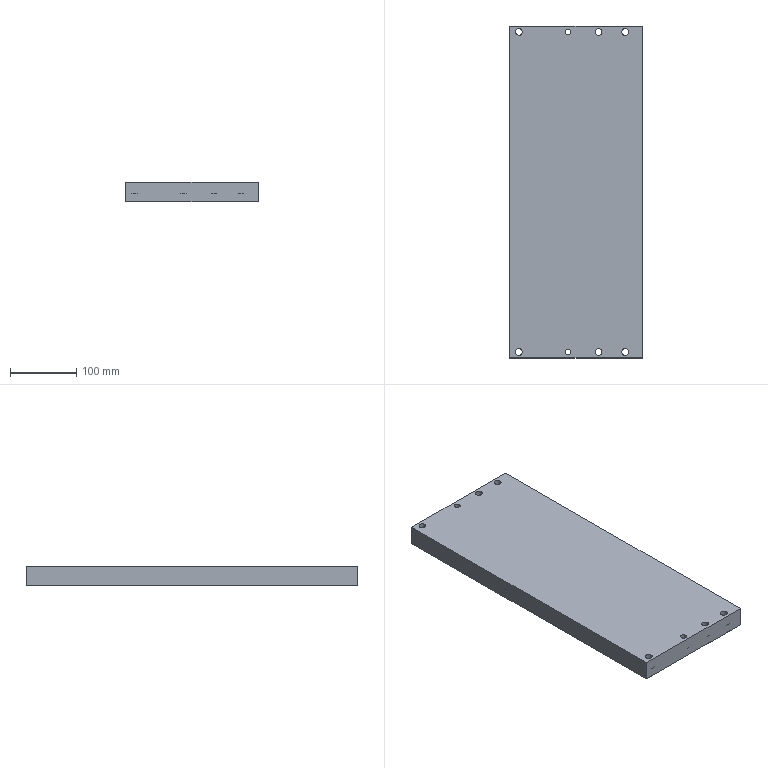Part | NX | 1 solid | 30 faces | box 200 x 500 x 30 mm | volume 2965920 mm3 | cylinder 16 | plane 14 | commonest cylinder face diameters 17 x8 10.3 x6 8.6 x2
STEP:
#1=CARTESIAN_POINT('',(-86.,-483.5,-60.));
#2=VERTEX_POINT('',#1);
#3=CARTESIAN_POINT('',(-86.,-492.,-60.));
#4=DIRECTION('',(0.,0.,-1.));
#5=DIRECTION('',(0.,1.,0.));
#6=AXIS2_PLACEMENT_3D('',#3,#4,#5);
#7=CIRCLE('',#6,8.5);
#8=EDGE_CURVE('',#2,#2,#7,.T.);
#9=ORIENTED_EDGE('',*,*,#8,.F.);
#10=EDGE_LOOP('',(#9));
#11=FACE_BOUND('',#10,.T.);
#12=CARTESIAN_POINT('',(-94.5,-492.,-73.));
#13=VERTEX_POINT('',#12);
#14=CARTESIAN_POINT('',(-86.,-492.,-73.));
#15=DIRECTION('',(0.,0.,-1.));
#16=DIRECTION('',(-1.,0.,0.));
#17=AXIS2_PLACEMENT_3D('',#14,#15,#16);
#18=CIRCLE('',#17,8.5);
#19=EDGE_CURVE('',#13,#13,#18,.F.);
#20=ORIENTED_EDGE('',*,*,#19,.F.);
#21=EDGE_LOOP('',(#20));
#22=FACE_BOUND('',#21,.T.);
#23=CARTESIAN_POINT('',(-86.,-492.,-60.));
#24=DIRECTION('',(0.,0.,-1.));
#25=DIRECTION('',(-1.,0.,0.));
#26=AXIS2_PLACEMENT_3D('',#23,#24,#25);
#27=CYLINDRICAL_SURFACE('',#26,8.5);
#28=ADVANCED_FACE('',(#11,#22),#27,.F.);
#29=ORIENTED_EDGE('',*,*,#8,.T.);
#30=EDGE_LOOP('',(#29));
#31=FACE_BOUND('',#30,.T.);
#32=CARTESIAN_POINT('',(-80.85,-492.,-60.));
#33=VERTEX_POINT('',#32);
#34=CARTESIAN_POINT('',(-86.,-492.,-60.));
#35=DIRECTION('',(0.,0.,-1.));
#36=DIRECTION('',(1.,0.,0.));
#37=AXIS2_PLACEMENT_3D('',#34,#35,#36);
#38=CIRCLE('',#37,5.15);
#39=EDGE_CURVE('',#33,#33,#38,.T.);
#40=ORIENTED_EDGE('',*,*,#39,.F.);
#41=EDGE_LOOP('',(#40));
#42=FACE_BOUND('',#41,.T.);
#43=CARTESIAN_POINT('',(-86.,-492.,-60.));
#44=DIRECTION('',(0.,0.,1.));
#45=DIRECTION('',(1.,0.,0.));
#46=AXIS2_PLACEMENT_3D('',#43,#44,#45);
#47=PLANE('',#46);
#48=ADVANCED_FACE('',(#31,#42),#47,.F.);
#49=ORIENTED_EDGE('',*,*,#39,.T.);
#50=EDGE_LOOP('',(#49));
#51=FACE_BOUND('',#50,.T.);
#52=CARTESIAN_POINT('',(-80.85,-492.,-43.));
#53=VERTEX_POINT('',#52);
#54=CARTESIAN_POINT('',(-86.,-492.,-43.));
#55=DIRECTION('',(0.,0.,1.));
#56=DIRECTION('',(1.,0.,0.));
#57=AXIS2_PLACEMENT_3D('',#54,#55,#56);
#58=CIRCLE('',#57,5.15);
#59=EDGE_CURVE('',#53,#53,#58,.T.);
#60=ORIENTED_EDGE('',*,*,#59,.T.);
#61=EDGE_LOOP('',(#60));
#62=FACE_BOUND('',#61,.T.);
#63=CARTESIAN_POINT('',(-86.,-492.,-78.));
#64=DIRECTION('',(0.,0.,1.));
#65=DIRECTION('',(1.,0.,0.));
#66=AXIS2_PLACEMENT_3D('',#63,#64,#65);
#67=CYLINDRICAL_SURFACE('',#66,5.15);
#68=ADVANCED_FACE('',(#51,#62),#67,.F.);
#69=CARTESIAN_POINT('',(79.15,-492.,-43.));
#70=VERTEX_POINT('',#69);
#71=CARTESIAN_POINT('',(74.,-492.,-43.));
#72=DIRECTION('',(0.,0.,1.));
#73=DIRECTION('',(1.,0.,0.));
#74=AXIS2_PLACEMENT_3D('',#71,#72,#73);
#75=CIRCLE('',#74,5.15);
#76=EDGE_CURVE('',#70,#70,#75,.F.);
#77=ORIENTED_EDGE('',*,*,#76,.F.);
#78=EDGE_LOOP('',(#77));
#79=FACE_BOUND('',#78,.T.);
#80=CARTESIAN_POINT('',(68.85,-492.,-60.));
#81=VERTEX_POINT('',#80);
#82=CARTESIAN_POINT('',(74.,-492.,-60.));
#83=DIRECTION('',(0.,0.,1.));
#84=DIRECTION('',(-1.,0.,0.));
#85=AXIS2_PLACEMENT_3D('',#82,#83,#84);
#86=CIRCLE('',#85,5.15);
#87=EDGE_CURVE('',#81,#81,#86,.F.);
#88=ORIENTED_EDGE('',*,*,#87,.T.);
#89=EDGE_LOOP('',(#88));
#90=FACE_BOUND('',#89,.T.);
#91=CARTESIAN_POINT('',(74.,-492.,-78.));
#92=DIRECTION('',(0.,0.,1.));
#93=DIRECTION('',(1.,0.,0.));
#94=AXIS2_PLACEMENT_3D('',#91,#92,#93);
#95=CYLINDRICAL_SURFACE('',#94,5.15);
#96=ADVANCED_FACE('',(#79,#90),#95,.F.);
#97=ORIENTED_EDGE('',*,*,#87,.F.);
#98=EDGE_LOOP('',(#97));
#99=FACE_BOUND('',#98,.T.);
#100=CARTESIAN_POINT('',(74.,-483.5,-60.));
#101=VERTEX_POINT('',#100);
#102=CARTESIAN_POINT('',(74.,-492.,-60.));
#103=DIRECTION('',(0.,0.,1.));
#104=DIRECTION('',(0.,1.,0.));
#105=AXIS2_PLACEMENT_3D('',#102,#103,#104);
#106=CIRCLE('',#105,8.5);
#107=EDGE_CURVE('',#101,#101,#106,.T.);
#108=ORIENTED_EDGE('',*,*,#107,.F.);
#109=EDGE_LOOP('',(#108));
#110=FACE_BOUND('',#109,.T.);
#111=CARTESIAN_POINT('',(74.,-492.,-60.));
#112=DIRECTION('',(0.,0.,-1.));
#113=DIRECTION('',(-1.,0.,0.));
#114=AXIS2_PLACEMENT_3D('',#111,#112,#113);
#115=PLANE('',#114);
#116=ADVANCED_FACE('',(#99,#110),#115,.T.);
#117=ORIENTED_EDGE('',*,*,#107,.T.);
#118=EDGE_LOOP('',(#117));
#119=FACE_BOUND('',#118,.T.);
#120=CARTESIAN_POINT('',(65.5,-492.,-73.));
#121=VERTEX_POINT('',#120);
#122=CARTESIAN_POINT('',(74.,-492.,-73.));
#123=DIRECTION('',(0.,0.,-1.));
#124=DIRECTION('',(-1.,0.,0.));
#125=AXIS2_PLACEMENT_3D('',#122,#123,#124);
#126=CIRCLE('',#125,8.5);
#127=EDGE_CURVE('',#121,#121,#126,.T.);
#128=ORIENTED_EDGE('',*,*,#127,.T.);
#129=EDGE_LOOP('',(#128));
#130=FACE_BOUND('',#129,.T.);
#131=CARTESIAN_POINT('',(74.,-492.,-60.));
#132=DIRECTION('',(0.,0.,-1.));
#133=DIRECTION('',(-1.,0.,0.));
#134=AXIS2_PLACEMENT_3D('',#131,#132,#133);
#135=CYLINDRICAL_SURFACE('',#134,8.5);
#136=ADVANCED_FACE('',(#119,#130),#135,.F.);
#137=CARTESIAN_POINT('',(39.15,-492.,-43.));
#138=VERTEX_POINT('',#137);
#139=CARTESIAN_POINT('',(34.,-492.,-43.));
#140=DIRECTION('',(0.,0.,1.));
#141=DIRECTION('',(1.,0.,0.));
#142=AXIS2_PLACEMENT_3D('',#139,#140,#141);
#143=CIRCLE('',#142,5.15);
#144=EDGE_CURVE('',#138,#138,#143,.F.);
#145=ORIENTED_EDGE('',*,*,#144,.F.);
#146=EDGE_LOOP('',(#145));
#147=FACE_BOUND('',#146,.T.);
#148=CARTESIAN_POINT('',(28.85,-492.,-60.));
#149=VERTEX_POINT('',#148);
#150=CARTESIAN_POINT('',(34.,-492.,-60.));
#151=DIRECTION('',(0.,0.,1.));
#152=DIRECTION('',(-1.,0.,0.));
#153=AXIS2_PLACEMENT_3D('',#150,#151,#152);
#154=CIRCLE('',#153,5.15);
#155=EDGE_CURVE('',#149,#149,#154,.F.);
#156=ORIENTED_EDGE('',*,*,#155,.T.);
#157=EDGE_LOOP('',(#156));
#158=FACE_BOUND('',#157,.T.);
#159=CARTESIAN_POINT('',(34.,-492.,-78.));
#160=DIRECTION('',(0.,0.,1.));
#161=DIRECTION('',(1.,0.,0.));
#162=AXIS2_PLACEMENT_3D('',#159,#160,#161);
#163=CYLINDRICAL_SURFACE('',#162,5.15);
#164=ADVANCED_FACE('',(#147,#158),#163,.F.);
#165=ORIENTED_EDGE('',*,*,#155,.F.);
#166=EDGE_LOOP('',(#165));
#167=FACE_BOUND('',#166,.T.);
#168=CARTESIAN_POINT('',(34.,-483.5,-60.));
#169=VERTEX_POINT('',#168);
#170=CARTESIAN_POINT('',(34.,-492.,-60.));
#171=DIRECTION('',(0.,0.,1.));
#172=DIRECTION('',(0.,1.,0.));
#173=AXIS2_PLACEMENT_3D('',#170,#171,#172);
#174=CIRCLE('',#173,8.5);
#175=EDGE_CURVE('',#169,#169,#174,.T.);
#176=ORIENTED_EDGE('',*,*,#175,.F.);
#177=EDGE_LOOP('',(#176));
#178=FACE_BOUND('',#177,.T.);
#179=CARTESIAN_POINT('',(34.,-492.,-60.));
#180=DIRECTION('',(0.,0.,-1.));
#181=DIRECTION('',(-1.,0.,0.));
#182=AXIS2_PLACEMENT_3D('',#179,#180,#181);
#183=PLANE('',#182);
#184=ADVANCED_FACE('',(#167,#178),#183,.T.);
#185=ORIENTED_EDGE('',*,*,#175,.T.);
#186=EDGE_LOOP('',(#185));
#187=FACE_BOUND('',#186,.T.);
#188=CARTESIAN_POINT('',(25.5,-492.,-73.));
#189=VERTEX_POINT('',#188);
#190=CARTESIAN_POINT('',(34.,-492.,-73.));
#191=DIRECTION('',(0.,0.,-1.));
#192=DIRECTION('',(-1.,0.,0.));
#193=AXIS2_PLACEMENT_3D('',#190,#191,#192);
#194=CIRCLE('',#193,8.5);
#195=EDGE_CURVE('',#189,#189,#194,.T.);
#196=ORIENTED_EDGE('',*,*,#195,.T.);
#197=EDGE_LOOP('',(#196));
#198=FACE_BOUND('',#197,.T.);
#199=CARTESIAN_POINT('',(34.,-492.,-60.));
#200=DIRECTION('',(0.,0.,-1.));
#201=DIRECTION('',(-1.,0.,0.));
#202=AXIS2_PLACEMENT_3D('',#199,#200,#201);
#203=CYLINDRICAL_SURFACE('',#202,8.5);
#204=ADVANCED_FACE('',(#187,#198),#203,.F.);
#205=CARTESIAN_POINT('',(-7.7,-492.,-43.));
#206=VERTEX_POINT('',#205);
#207=CARTESIAN_POINT('',(-12.,-492.,-43.));
#208=DIRECTION('',(0.,0.,1.));
#209=DIRECTION('',(1.,0.,0.));
#210=AXIS2_PLACEMENT_3D('',#207,#208,#209);
#211=CIRCLE('',#210,4.3);
#212=EDGE_CURVE('',#206,#206,#211,.F.);
#213=ORIENTED_EDGE('',*,*,#212,.F.);
#214=EDGE_LOOP('',(#213));
#215=FACE_BOUND('',#214,.T.);
#216=CARTESIAN_POINT('',(-16.3,-492.,-60.));
#217=VERTEX_POINT('',#216);
#218=CARTESIAN_POINT('',(-12.,-492.,-60.));
#219=DIRECTION('',(0.,0.,1.));
#220=DIRECTION('',(-1.,0.,0.));
#221=AXIS2_PLACEMENT_3D('',#218,#219,#220);
#222=CIRCLE('',#221,4.3);
#223=EDGE_CURVE('',#217,#217,#222,.F.);
#224=ORIENTED_EDGE('',*,*,#223,.T.);
#225=EDGE_LOOP('',(#224));
#226=FACE_BOUND('',#225,.T.);
#227=CARTESIAN_POINT('',(-12.,-492.,-78.));
#228=DIRECTION('',(0.,0.,1.));
#229=DIRECTION('',(1.,0.,0.));
#230=AXIS2_PLACEMENT_3D('',#227,#228,#229);
#231=CYLINDRICAL_SURFACE('',#230,4.3);
#232=ADVANCED_FACE('',(#215,#226),#231,.F.);
#233=ORIENTED_EDGE('',*,*,#223,.F.);
#234=EDGE_LOOP('',(#233));
#235=FACE_BOUND('',#234,.T.);
#236=CARTESIAN_POINT('',(-12.,-483.5,-60.));
#237=VERTEX_POINT('',#236);
#238=CARTESIAN_POINT('',(-12.,-492.,-60.));
#239=DIRECTION('',(0.,0.,1.));
#240=DIRECTION('',(0.,1.,0.));
#241=AXIS2_PLACEMENT_3D('',#238,#239,#240);
#242=CIRCLE('',#241,8.5);
#243=EDGE_CURVE('',#237,#237,#242,.T.);
#244=ORIENTED_EDGE('',*,*,#243,.F.);
#245=EDGE_LOOP('',(#244));
#246=FACE_BOUND('',#245,.T.);
#247=CARTESIAN_POINT('',(-12.,-492.,-60.));
#248=DIRECTION('',(0.,0.,-1.));
#249=DIRECTION('',(-1.,0.,0.));
#250=AXIS2_PLACEMENT_3D('',#247,#248,#249);
#251=PLANE('',#250);
#252=ADVANCED_FACE('',(#235,#246),#251,.T.);
#253=ORIENTED_EDGE('',*,*,#243,.T.);
#254=EDGE_LOOP('',(#253));
#255=FACE_BOUND('',#254,.T.);
#256=CARTESIAN_POINT('',(-20.5,-492.,-73.));
#257=VERTEX_POINT('',#256);
#258=CARTESIAN_POINT('',(-12.,-492.,-73.));
#259=DIRECTION('',(0.,0.,-1.));
#260=DIRECTION('',(-1.,0.,0.));
#261=AXIS2_PLACEMENT_3D('',#258,#259,#260);
#262=CIRCLE('',#261,8.5);
#263=EDGE_CURVE('',#257,#257,#262,.T.);
#264=ORIENTED_EDGE('',*,*,#263,.T.);
#265=EDGE_LOOP('',(#264));
#266=FACE_BOUND('',#265,.T.);
#267=CARTESIAN_POINT('',(-12.,-492.,-60.));
#268=DIRECTION('',(0.,0.,-1.));
#269=DIRECTION('',(-1.,0.,0.));
#270=AXIS2_PLACEMENT_3D('',#267,#268,#269);
#271=CYLINDRICAL_SURFACE('',#270,8.5);
#272=ADVANCED_FACE('',(#255,#266),#271,.F.);
#273=CARTESIAN_POINT('',(28.85,-10.,-60.));
#274=VERTEX_POINT('',#273);
#275=CARTESIAN_POINT('',(34.,-10.,-60.));
#276=DIRECTION('',(0.,0.,-1.));
#277=DIRECTION('',(-1.,0.,0.));
#278=AXIS2_PLACEMENT_3D('',#275,#276,#277);
#279=CIRCLE('',#278,5.15);
#280=EDGE_CURVE('',#274,#274,#279,.T.);
#281=ORIENTED_EDGE('',*,*,#280,.F.);
#282=EDGE_LOOP('',(#281));
#283=FACE_BOUND('',#282,.T.);
#284=CARTESIAN_POINT('',(34.,-18.5,-60.));
#285=VERTEX_POINT('',#284);
#286=CARTESIAN_POINT('',(34.,-10.,-60.));
#287=DIRECTION('',(0.,0.,-1.));
#288=DIRECTION('',(0.,-1.,0.));
#289=AXIS2_PLACEMENT_3D('',#286,#287,#288);
#290=CIRCLE('',#289,8.5);
#291=EDGE_CURVE('',#285,#285,#290,.F.);
#292=ORIENTED_EDGE('',*,*,#291,.F.);
#293=EDGE_LOOP('',(#292));
#294=FACE_BOUND('',#293,.T.);
#295=CARTESIAN_POINT('',(34.,-10.,-60.));
#296=DIRECTION('',(0.,0.,-1.));
#297=DIRECTION('',(-1.,0.,0.));
#298=AXIS2_PLACEMENT_3D('',#295,#296,#297);
#299=PLANE('',#298);
#300=ADVANCED_FACE('',(#283,#294),#299,.T.);
#301=CARTESIAN_POINT('',(-86.,-18.5,-60.));
#302=VERTEX_POINT('',#301);
#303=CARTESIAN_POINT('',(-86.,-10.,-60.));
#304=DIRECTION('',(0.,0.,1.));
#305=DIRECTION('',(0.,-1.,0.));
#306=AXIS2_PLACEMENT_3D('',#303,#304,#305);
#307=CIRCLE('',#306,8.5);
#308=EDGE_CURVE('',#302,#302,#307,.F.);
#309=ORIENTED_EDGE('',*,*,#308,.T.);
#310=EDGE_LOOP('',(#309));
#311=FACE_BOUND('',#310,.T.);
#312=CARTESIAN_POINT('',(-80.85,-10.,-60.));
#313=VERTEX_POINT('',#312);
#314=CARTESIAN_POINT('',(-86.,-10.,-60.));
#315=DIRECTION('',(0.,0.,1.));
#316=DIRECTION('',(1.,0.,0.));
#317=AXIS2_PLACEMENT_3D('',#314,#315,#316);
#318=CIRCLE('',#317,5.15);
#319=EDGE_CURVE('',#313,#313,#318,.F.);
#320=ORIENTED_EDGE('',*,*,#319,.F.);
#321=EDGE_LOOP('',(#320));
#322=FACE_BOUND('',#321,.T.);
#323=CARTESIAN_POINT('',(-86.,-10.,-60.));
#324=DIRECTION('',(0.,0.,1.));
#325=DIRECTION('',(1.,0.,0.));
#326=AXIS2_PLACEMENT_3D('',#323,#324,#325);
#327=PLANE('',#326);
#328=ADVANCED_FACE('',(#311,#322),#327,.F.);
#329=CARTESIAN_POINT('',(-16.3,-10.,-60.));
#330=VERTEX_POINT('',#329);
#331=CARTESIAN_POINT('',(-12.,-10.,-60.));
#332=DIRECTION('',(0.,0.,-1.));
#333=DIRECTION('',(-1.,0.,0.));
#334=AXIS2_PLACEMENT_3D('',#331,#332,#333);
#335=CIRCLE('',#334,4.3);
#336=EDGE_CURVE('',#330,#330,#335,.T.);
#337=ORIENTED_EDGE('',*,*,#336,.F.);
#338=EDGE_LOOP('',(#337));
#339=FACE_BOUND('',#338,.T.);
#340=CARTESIAN_POINT('',(-12.,-18.5,-60.));
#341=VERTEX_POINT('',#340);
#342=CARTESIAN_POINT('',(-12.,-10.,-60.));
#343=DIRECTION('',(0.,0.,-1.));
#344=DIRECTION('',(0.,-1.,0.));
#345=AXIS2_PLACEMENT_3D('',#342,#343,#344);
#346=CIRCLE('',#345,8.5);
#347=EDGE_CURVE('',#341,#341,#346,.F.);
#348=ORIENTED_EDGE('',*,*,#347,.F.);
#349=EDGE_LOOP('',(#348));
#350=FACE_BOUND('',#349,.T.);
#351=CARTESIAN_POINT('',(-12.,-10.,-60.));
#352=DIRECTION('',(0.,0.,-1.));
#353=DIRECTION('',(-1.,0.,0.));
#354=AXIS2_PLACEMENT_3D('',#351,#352,#353);
#355=PLANE('',#354);
#356=ADVANCED_FACE('',(#339,#350),#355,.T.);
#357=CARTESIAN_POINT('',(68.85,-10.,-60.));
#358=VERTEX_POINT('',#357);
#359=CARTESIAN_POINT('',(74.,-10.,-60.));
#360=DIRECTION('',(0.,0.,-1.));
#361=DIRECTION('',(-1.,0.,0.));
#362=AXIS2_PLACEMENT_3D('',#359,#360,#361);
#363=CIRCLE('',#362,5.15);
#364=EDGE_CURVE('',#358,#358,#363,.T.);
#365=ORIENTED_EDGE('',*,*,#364,.F.);
#366=EDGE_LOOP('',(#365));
#367=FACE_BOUND('',#366,.T.);
#368=CARTESIAN_POINT('',(74.,-18.5,-60.));
#369=VERTEX_POINT('',#368);
#370=CARTESIAN_POINT('',(74.,-10.,-60.));
#371=DIRECTION('',(0.,0.,-1.));
#372=DIRECTION('',(0.,-1.,0.));
#373=AXIS2_PLACEMENT_3D('',#370,#371,#372);
#374=CIRCLE('',#373,8.5);
#375=EDGE_CURVE('',#369,#369,#374,.F.);
#376=ORIENTED_EDGE('',*,*,#375,.F.);
#377=EDGE_LOOP('',(#376));
#378=FACE_BOUND('',#377,.T.);
#379=CARTESIAN_POINT('',(74.,-10.,-60.));
#380=DIRECTION('',(0.,0.,-1.));
#381=DIRECTION('',(-1.,0.,0.));
#382=AXIS2_PLACEMENT_3D('',#379,#380,#381);
#383=PLANE('',#382);
#384=ADVANCED_FACE('',(#367,#378),#383,.T.);
#385=CARTESIAN_POINT('',(79.15,-10.,-43.));
#386=VERTEX_POINT('',#385);
#387=CARTESIAN_POINT('',(74.,-10.,-43.));
#388=DIRECTION('',(0.,0.,1.));
#389=DIRECTION('',(1.,0.,0.));
#390=AXIS2_PLACEMENT_3D('',#387,#388,#389);
#391=CIRCLE('',#390,5.15);
#392=EDGE_CURVE('',#386,#386,#391,.F.);
#393=ORIENTED_EDGE('',*,*,#392,.F.);
#394=EDGE_LOOP('',(#393));
#395=FACE_BOUND('',#394,.T.);
#396=ORIENTED_EDGE('',*,*,#364,.T.);
#397=EDGE_LOOP('',(#396));
#398=FACE_BOUND('',#397,.T.);
#399=CARTESIAN_POINT('',(74.,-10.,-78.));
#400=DIRECTION('',(0.,0.,1.));
#401=DIRECTION('',(1.,0.,0.));
#402=AXIS2_PLACEMENT_3D('',#399,#400,#401);
#403=CYLINDRICAL_SURFACE('',#402,5.15);
#404=ADVANCED_FACE('',(#395,#398),#403,.F.);
#405=CARTESIAN_POINT('',(39.15,-10.,-43.));
#406=VERTEX_POINT('',#405);
#407=CARTESIAN_POINT('',(34.,-10.,-43.));
#408=DIRECTION('',(0.,0.,1.));
#409=DIRECTION('',(1.,0.,0.));
#410=AXIS2_PLACEMENT_3D('',#407,#408,#409);
#411=CIRCLE('',#410,5.15);
#412=EDGE_CURVE('',#406,#406,#411,.F.);
#413=ORIENTED_EDGE('',*,*,#412,.F.);
#414=EDGE_LOOP('',(#413));
#415=FACE_BOUND('',#414,.T.);
#416=ORIENTED_EDGE('',*,*,#280,.T.);
#417=EDGE_LOOP('',(#416));
#418=FACE_BOUND('',#417,.T.);
#419=CARTESIAN_POINT('',(34.,-10.,-78.));
#420=DIRECTION('',(0.,0.,1.));
#421=DIRECTION('',(1.,0.,0.));
#422=AXIS2_PLACEMENT_3D('',#419,#420,#421);
#423=CYLINDRICAL_SURFACE('',#422,5.15);
#424=ADVANCED_FACE('',(#415,#418),#423,.F.);
#425=CARTESIAN_POINT('',(-7.7,-10.,-43.));
#426=VERTEX_POINT('',#425);
#427=CARTESIAN_POINT('',(-12.,-10.,-43.));
#428=DIRECTION('',(0.,0.,1.));
#429=DIRECTION('',(1.,0.,0.));
#430=AXIS2_PLACEMENT_3D('',#427,#428,#429);
#431=CIRCLE('',#430,4.3);
#432=EDGE_CURVE('',#426,#426,#431,.F.);
#433=ORIENTED_EDGE('',*,*,#432,.F.);
#434=EDGE_LOOP('',(#433));
#435=FACE_BOUND('',#434,.T.);
#436=ORIENTED_EDGE('',*,*,#336,.T.);
#437=EDGE_LOOP('',(#436));
#438=FACE_BOUND('',#437,.T.);
#439=CARTESIAN_POINT('',(-12.,-10.,-78.));
#440=DIRECTION('',(0.,0.,1.));
#441=DIRECTION('',(1.,0.,0.));
#442=AXIS2_PLACEMENT_3D('',#439,#440,#441);
#443=CYLINDRICAL_SURFACE('',#442,4.3);
#444=ADVANCED_FACE('',(#435,#438),#443,.F.);
#445=ORIENTED_EDGE('',*,*,#319,.T.);
#446=EDGE_LOOP('',(#445));
#447=FACE_BOUND('',#446,.T.);
#448=CARTESIAN_POINT('',(-86.,-15.15,-43.));
#449=VERTEX_POINT('',#448);
#450=CARTESIAN_POINT('',(-86.,-10.,-43.));
#451=DIRECTION('',(0.,0.,1.));
#452=DIRECTION('',(0.,-1.,0.));
#453=AXIS2_PLACEMENT_3D('',#450,#451,#452);
#454=CIRCLE('',#453,5.15);
#455=EDGE_CURVE('',#449,#449,#454,.T.);
#456=ORIENTED_EDGE('',*,*,#455,.T.);
#457=EDGE_LOOP('',(#456));
#458=FACE_BOUND('',#457,.T.);
#459=CARTESIAN_POINT('',(-86.,-10.,-78.));
#460=DIRECTION('',(0.,0.,1.));
#461=DIRECTION('',(1.,0.,0.));
#462=AXIS2_PLACEMENT_3D('',#459,#460,#461);
#463=CYLINDRICAL_SURFACE('',#462,5.15);
#464=ADVANCED_FACE('',(#447,#458),#463,.F.);
#465=CARTESIAN_POINT('',(-100.,-1.,-73.));
#466=VERTEX_POINT('',#465);
#467=CARTESIAN_POINT('',(-100.,-1.,-43.));
#468=VERTEX_POINT('',#467);
#469=CARTESIAN_POINT('',(-100.,-1.,-73.));
#470=DIRECTION('',(0.,0.,1.));
#471=VECTOR('',#470,1000.);
#472=LINE('',#469,#471);
#473=EDGE_CURVE('',#466,#468,#472,.T.);
#474=ORIENTED_EDGE('',*,*,#473,.T.);
#475=CARTESIAN_POINT('',(100.,-1.,-43.));
#476=VERTEX_POINT('',#475);
#477=CARTESIAN_POINT('',(0.,-1.,-43.));
#478=DIRECTION('',(1.,0.,0.));
#479=VECTOR('',#478,1000.);
#480=LINE('',#477,#479);
#481=EDGE_CURVE('',#468,#476,#480,.T.);
#482=ORIENTED_EDGE('',*,*,#481,.T.);
#483=CARTESIAN_POINT('',(100.,-1.,-73.));
#484=VERTEX_POINT('',#483);
#485=CARTESIAN_POINT('',(100.,-1.,-73.));
#486=DIRECTION('',(0.,0.,1.));
#487=VECTOR('',#486,1000.);
#488=LINE('',#485,#487);
#489=EDGE_CURVE('',#484,#476,#488,.T.);
#490=ORIENTED_EDGE('',*,*,#489,.F.);
#491=CARTESIAN_POINT('',(0.,-1.,-73.));
#492=DIRECTION('',(-1.,0.,0.));
#493=VECTOR('',#492,1000.);
#494=LINE('',#491,#493);
#495=EDGE_CURVE('',#484,#466,#494,.T.);
#496=ORIENTED_EDGE('',*,*,#495,.T.);
#497=EDGE_LOOP('',(#474,#482,#490,#496));
#498=FACE_BOUND('',#497,.T.);
#499=CARTESIAN_POINT('',(0.,-1.,-73.));
#500=DIRECTION('',(0.,1.,0.));
#501=DIRECTION('',(0.,0.,1.));
#502=AXIS2_PLACEMENT_3D('',#499,#500,#501);
#503=PLANE('',#502);
#504=ADVANCED_FACE('',(#498),#503,.T.);
#505=CARTESIAN_POINT('',(-100.,-501.,-73.));
#506=VERTEX_POINT('',#505);
#507=CARTESIAN_POINT('',(-100.,-501.,-43.));
#508=VERTEX_POINT('',#507);
#509=CARTESIAN_POINT('',(-100.,-501.,-73.));
#510=DIRECTION('',(0.,0.,1.));
#511=VECTOR('',#510,1000.);
#512=LINE('',#509,#511);
#513=EDGE_CURVE('',#506,#508,#512,.T.);
#514=ORIENTED_EDGE('',*,*,#513,.T.);
#515=CARTESIAN_POINT('',(-100.,-251.,-43.));
#516=DIRECTION('',(0.,1.,0.));
#517=VECTOR('',#516,1000.);
#518=LINE('',#515,#517);
#519=EDGE_CURVE('',#508,#468,#518,.T.);
#520=ORIENTED_EDGE('',*,*,#519,.T.);
#521=ORIENTED_EDGE('',*,*,#473,.F.);
#522=CARTESIAN_POINT('',(-100.,-251.,-73.));
#523=DIRECTION('',(0.,-1.,0.));
#524=VECTOR('',#523,1000.);
#525=LINE('',#522,#524);
#526=EDGE_CURVE('',#466,#506,#525,.T.);
#527=ORIENTED_EDGE('',*,*,#526,.T.);
#528=EDGE_LOOP('',(#514,#520,#521,#527));
#529=FACE_BOUND('',#528,.T.);
#530=CARTESIAN_POINT('',(-100.,-251.,-73.));
#531=DIRECTION('',(-1.,0.,0.));
#532=DIRECTION('',(0.,0.,1.));
#533=AXIS2_PLACEMENT_3D('',#530,#531,#532);
#534=PLANE('',#533);
#535=ADVANCED_FACE('',(#529),#534,.T.);
#536=CARTESIAN_POINT('',(100.,-501.,-73.));
#537=VERTEX_POINT('',#536);
#538=CARTESIAN_POINT('',(100.,-501.,-43.));
#539=VERTEX_POINT('',#538);
#540=CARTESIAN_POINT('',(100.,-501.,-73.));
#541=DIRECTION('',(0.,0.,1.));
#542=VECTOR('',#541,1000.);
#543=LINE('',#540,#542);
#544=EDGE_CURVE('',#537,#539,#543,.T.);
#545=ORIENTED_EDGE('',*,*,#544,.T.);
#546=CARTESIAN_POINT('',(0.,-501.,-43.));
#547=DIRECTION('',(-1.,0.,0.));
#548=VECTOR('',#547,1000.);
#549=LINE('',#546,#548);
#550=EDGE_CURVE('',#539,#508,#549,.T.);
#551=ORIENTED_EDGE('',*,*,#550,.T.);
#552=ORIENTED_EDGE('',*,*,#513,.F.);
#553=CARTESIAN_POINT('',(0.,-501.,-73.));
#554=DIRECTION('',(1.,0.,0.));
#555=VECTOR('',#554,1000.);
#556=LINE('',#553,#555);
#557=EDGE_CURVE('',#506,#537,#556,.T.);
#558=ORIENTED_EDGE('',*,*,#557,.T.);
#559=EDGE_LOOP('',(#545,#551,#552,#558));
#560=FACE_BOUND('',#559,.T.);
#561=CARTESIAN_POINT('',(0.,-501.,-73.));
#562=DIRECTION('',(0.,-1.,0.));
#563=DIRECTION('',(0.,0.,-1.));
#564=AXIS2_PLACEMENT_3D('',#561,#562,#563);
#565=PLANE('',#564);
#566=ADVANCED_FACE('',(#560),#565,.T.);
#567=CARTESIAN_POINT('',(100.,-251.,-73.));
#568=DIRECTION('',(0.,1.,0.));
#569=VECTOR('',#568,1000.);
#570=LINE('',#567,#569);
#571=EDGE_CURVE('',#537,#484,#570,.T.);
#572=ORIENTED_EDGE('',*,*,#571,.T.);
#573=ORIENTED_EDGE('',*,*,#489,.T.);
#574=CARTESIAN_POINT('',(100.,-251.,-43.));
#575=DIRECTION('',(0.,-1.,0.));
#576=VECTOR('',#575,1000.);
#577=LINE('',#574,#576);
#578=EDGE_CURVE('',#476,#539,#577,.T.);
#579=ORIENTED_EDGE('',*,*,#578,.T.);
#580=ORIENTED_EDGE('',*,*,#544,.F.);
#581=EDGE_LOOP('',(#572,#573,#579,#580));
#582=FACE_BOUND('',#581,.T.);
#583=CARTESIAN_POINT('',(100.,-251.,-73.));
#584=DIRECTION('',(1.,0.,0.));
#585=DIRECTION('',(0.,0.,-1.));
#586=AXIS2_PLACEMENT_3D('',#583,#584,#585);
#587=PLANE('',#586);
#588=ADVANCED_FACE('',(#582),#587,.T.);
#589=ORIENTED_EDGE('',*,*,#291,.T.);
#590=EDGE_LOOP('',(#589));
#591=FACE_BOUND('',#590,.T.);
#592=CARTESIAN_POINT('',(34.,-18.5,-73.));
#593=VERTEX_POINT('',#592);
#594=CARTESIAN_POINT('',(34.,-10.,-73.));
#595=DIRECTION('',(0.,0.,-1.));
#596=DIRECTION('',(0.,-1.,0.));
#597=AXIS2_PLACEMENT_3D('',#594,#595,#596);
#598=CIRCLE('',#597,8.5);
#599=EDGE_CURVE('',#593,#593,#598,.T.);
#600=ORIENTED_EDGE('',*,*,#599,.T.);
#601=EDGE_LOOP('',(#600));
#602=FACE_BOUND('',#601,.T.);
#603=CARTESIAN_POINT('',(34.,-10.,-60.));
#604=DIRECTION('',(0.,0.,-1.));
#605=DIRECTION('',(-1.,0.,0.));
#606=AXIS2_PLACEMENT_3D('',#603,#604,#605);
#607=CYLINDRICAL_SURFACE('',#606,8.5);
#608=ADVANCED_FACE('',(#591,#602),#607,.F.);
#609=ORIENTED_EDGE('',*,*,#308,.F.);
#610=EDGE_LOOP('',(#609));
#611=FACE_BOUND('',#610,.T.);
#612=CARTESIAN_POINT('',(-86.,-18.5,-73.));
#613=VERTEX_POINT('',#612);
#614=CARTESIAN_POINT('',(-86.,-10.,-73.));
#615=DIRECTION('',(0.,0.,1.));
#616=DIRECTION('',(0.,-1.,0.));
#617=AXIS2_PLACEMENT_3D('',#614,#615,#616);
#618=CIRCLE('',#617,8.5);
#619=EDGE_CURVE('',#613,#613,#618,.T.);
#620=ORIENTED_EDGE('',*,*,#619,.F.);
#621=EDGE_LOOP('',(#620));
#622=FACE_BOUND('',#621,.T.);
#623=CARTESIAN_POINT('',(-86.,-10.,-60.));
#624=DIRECTION('',(0.,0.,-1.));
#625=DIRECTION('',(-1.,0.,0.));
#626=AXIS2_PLACEMENT_3D('',#623,#624,#625);
#627=CYLINDRICAL_SURFACE('',#626,8.5);
#628=ADVANCED_FACE('',(#611,#622),#627,.F.);
#629=ORIENTED_EDGE('',*,*,#347,.T.);
#630=EDGE_LOOP('',(#629));
#631=FACE_BOUND('',#630,.T.);
#632=CARTESIAN_POINT('',(-12.,-18.5,-73.));
#633=VERTEX_POINT('',#632);
#634=CARTESIAN_POINT('',(-12.,-10.,-73.));
#635=DIRECTION('',(0.,0.,-1.));
#636=DIRECTION('',(0.,-1.,0.));
#637=AXIS2_PLACEMENT_3D('',#634,#635,#636);
#638=CIRCLE('',#637,8.5);
#639=EDGE_CURVE('',#633,#633,#638,.T.);
#640=ORIENTED_EDGE('',*,*,#639,.T.);
#641=EDGE_LOOP('',(#640));
#642=FACE_BOUND('',#641,.T.);
#643=CARTESIAN_POINT('',(-12.,-10.,-60.));
#644=DIRECTION('',(0.,0.,-1.));
#645=DIRECTION('',(-1.,0.,0.));
#646=AXIS2_PLACEMENT_3D('',#643,#644,#645);
#647=CYLINDRICAL_SURFACE('',#646,8.5);
#648=ADVANCED_FACE('',(#631,#642),#647,.F.);
#649=ORIENTED_EDGE('',*,*,#375,.T.);
#650=EDGE_LOOP('',(#649));
#651=FACE_BOUND('',#650,.T.);
#652=CARTESIAN_POINT('',(74.,-18.5,-73.));
#653=VERTEX_POINT('',#652);
#654=CARTESIAN_POINT('',(74.,-10.,-73.));
#655=DIRECTION('',(0.,0.,-1.));
#656=DIRECTION('',(0.,-1.,0.));
#657=AXIS2_PLACEMENT_3D('',#654,#655,#656);
#658=CIRCLE('',#657,8.5);
#659=EDGE_CURVE('',#653,#653,#658,.T.);
#660=ORIENTED_EDGE('',*,*,#659,.T.);
#661=EDGE_LOOP('',(#660));
#662=FACE_BOUND('',#661,.T.);
#663=CARTESIAN_POINT('',(74.,-10.,-60.));
#664=DIRECTION('',(0.,0.,-1.));
#665=DIRECTION('',(-1.,0.,0.));
#666=AXIS2_PLACEMENT_3D('',#663,#664,#665);
#667=CYLINDRICAL_SURFACE('',#666,8.5);
#668=ADVANCED_FACE('',(#651,#662),#667,.F.);
#669=ORIENTED_EDGE('',*,*,#19,.T.);
#670=EDGE_LOOP('',(#669));
#671=FACE_BOUND('',#670,.T.);
#672=ORIENTED_EDGE('',*,*,#659,.F.);
#673=EDGE_LOOP('',(#672));
#674=FACE_BOUND('',#673,.T.);
#675=ORIENTED_EDGE('',*,*,#639,.F.);
#676=EDGE_LOOP('',(#675));
#677=FACE_BOUND('',#676,.T.);
#678=ORIENTED_EDGE('',*,*,#619,.T.);
#679=EDGE_LOOP('',(#678));
#680=FACE_BOUND('',#679,.T.);
#681=ORIENTED_EDGE('',*,*,#599,.F.);
#682=EDGE_LOOP('',(#681));
#683=FACE_BOUND('',#682,.T.);
#684=ORIENTED_EDGE('',*,*,#571,.F.);
#685=ORIENTED_EDGE('',*,*,#557,.F.);
#686=ORIENTED_EDGE('',*,*,#526,.F.);
#687=ORIENTED_EDGE('',*,*,#495,.F.);
#688=EDGE_LOOP('',(#684,#685,#686,#687));
#689=FACE_BOUND('',#688,.T.);
#690=ORIENTED_EDGE('',*,*,#127,.F.);
#691=EDGE_LOOP('',(#690));
#692=FACE_BOUND('',#691,.T.);
#693=ORIENTED_EDGE('',*,*,#195,.F.);
#694=EDGE_LOOP('',(#693));
#695=FACE_BOUND('',#694,.T.);
#696=ORIENTED_EDGE('',*,*,#263,.F.);
#697=EDGE_LOOP('',(#696));
#698=FACE_BOUND('',#697,.T.);
#699=CARTESIAN_POINT('',(0.,-251.,-73.));
#700=DIRECTION('',(0.,0.,-1.));
#701=DIRECTION('',(-1.,0.,0.));
#702=AXIS2_PLACEMENT_3D('',#699,#700,#701);
#703=PLANE('',#702);
#704=ADVANCED_FACE('',(#671,#674,#677,#680,#683,#689,#692,#695,#698),#703,.T.);
#705=ORIENTED_EDGE('',*,*,#144,.T.);
#706=EDGE_LOOP('',(#705));
#707=FACE_BOUND('',#706,.T.);
#708=ORIENTED_EDGE('',*,*,#550,.F.);
#709=ORIENTED_EDGE('',*,*,#578,.F.);
#710=ORIENTED_EDGE('',*,*,#481,.F.);
#711=ORIENTED_EDGE('',*,*,#519,.F.);
#712=EDGE_LOOP('',(#708,#709,#710,#711));
#713=FACE_BOUND('',#712,.T.);
#714=ORIENTED_EDGE('',*,*,#455,.F.);
#715=EDGE_LOOP('',(#714));
#716=FACE_BOUND('',#715,.T.);
#717=ORIENTED_EDGE('',*,*,#432,.T.);
#718=EDGE_LOOP('',(#717));
#719=FACE_BOUND('',#718,.T.);
#720=ORIENTED_EDGE('',*,*,#412,.T.);
#721=EDGE_LOOP('',(#720));
#722=FACE_BOUND('',#721,.T.);
#723=ORIENTED_EDGE('',*,*,#392,.T.);
#724=EDGE_LOOP('',(#723));
#725=FACE_BOUND('',#724,.T.);
#726=ORIENTED_EDGE('',*,*,#59,.F.);
#727=EDGE_LOOP('',(#726));
#728=FACE_BOUND('',#727,.T.);
#729=ORIENTED_EDGE('',*,*,#76,.T.);
#730=EDGE_LOOP('',(#729));
#731=FACE_BOUND('',#730,.T.);
#732=ORIENTED_EDGE('',*,*,#212,.T.);
#733=EDGE_LOOP('',(#732));
#734=FACE_BOUND('',#733,.T.);
#735=CARTESIAN_POINT('',(0.,-251.,-43.));
#736=DIRECTION('',(0.,0.,1.));
#737=DIRECTION('',(1.,0.,0.));
#738=AXIS2_PLACEMENT_3D('',#735,#736,#737);
#739=PLANE('',#738);
#740=ADVANCED_FACE('',(#707,#713,#716,#719,#722,#725,#728,#731,#734),#739,.T.);
#741=CLOSED_SHELL('',(#28,#48,#68,#96,#116,#136,#164,#184,#204,#232,#252,#272,#300,#328,#356,#384,#404,#424,#444,#464,#504,#535,#566,#588,#608,#628,#648,#668,#704,#740));
#742=MANIFOLD_SOLID_BREP('',#741);
#743=(LENGTH_UNIT()NAMED_UNIT(*)SI_UNIT(.MILLI.,.METRE.));
#744=UNCERTAINTY_MEASURE_WITH_UNIT(LENGTH_MEASURE(0.00001),#743,'','');
#745=(NAMED_UNIT(*)PLANE_ANGLE_UNIT()SI_UNIT($,.RADIAN.));
#746=(NAMED_UNIT(*)SI_UNIT($,.STERADIAN.)SOLID_ANGLE_UNIT());
#747=(GEOMETRIC_REPRESENTATION_CONTEXT(3)GLOBAL_UNCERTAINTY_ASSIGNED_CONTEXT((#744))GLOBAL_UNIT_ASSIGNED_CONTEXT((#743,#745,#746))REPRESENTATION_CONTEXT('',''));
#748=ADVANCED_BREP_SHAPE_REPRESENTATION('',(#742),#747);